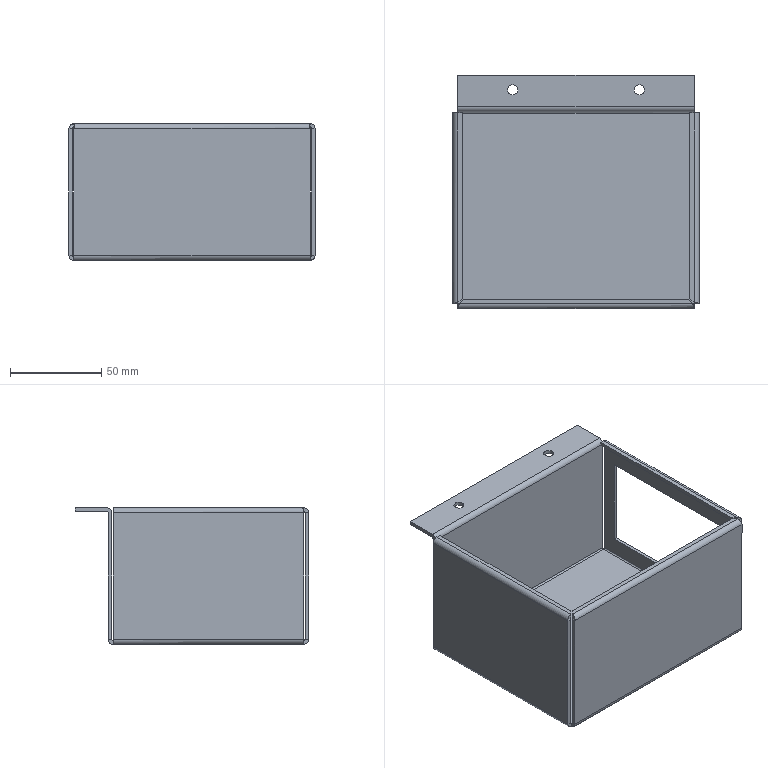Part | SolidWorks | features BaseBody 1 | 1 solid | 70 faces | box 135 x 128 x 75 mm | volume 94183 mm3 | plane 38 | cylinder 20 | spline 12 | commonest cylinder face diameters 1.473 x8 5.473 x8 5.5 x4